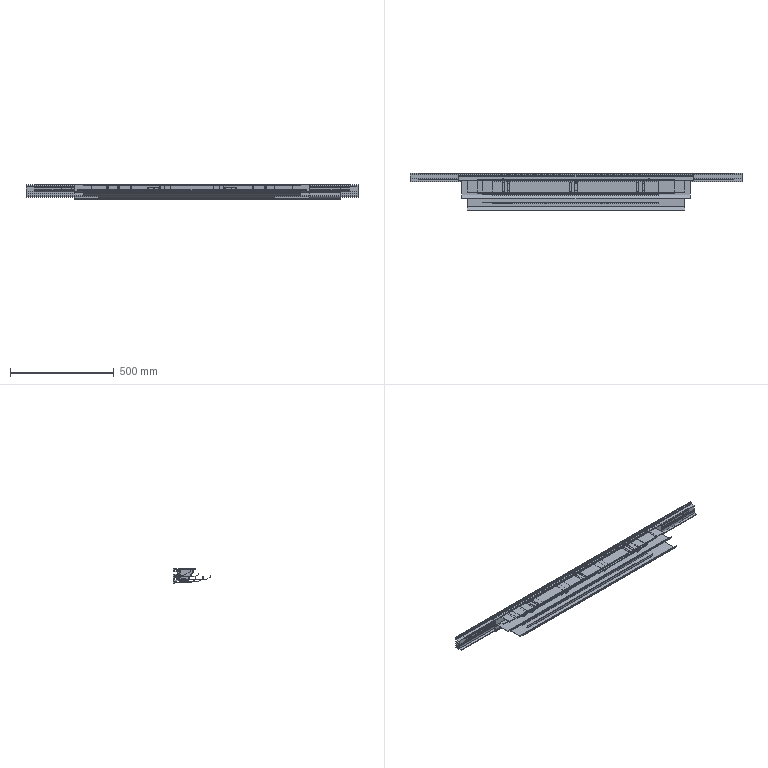Part | SolidWorks | 31 solids | 973 faces | box 1600 x 178.321 x 70 mm | volume 4811022 mm3 | plane 665 | cylinder 308 | commonest cylinder face diameters 10 x85 7 x45 9 x42 2 x37 6 x34 3 x18